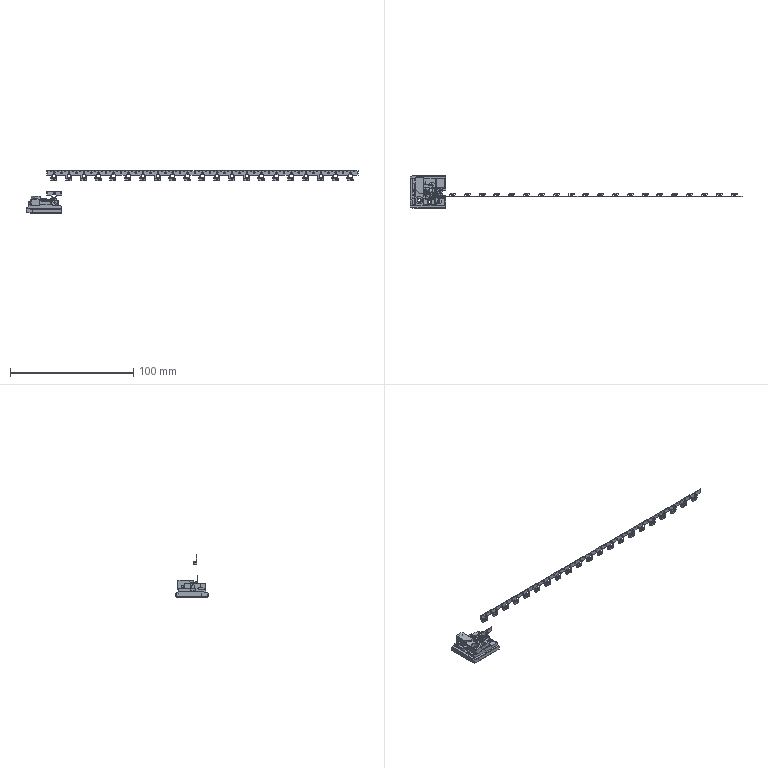Part | NX | 10 solids | 4586 faces | volume 5246 mm3 | plane 2703 | cylinder 1443 | torus 302 | spline 62 | sphere 48 | cone 28 | commonest cylinder face diameters 0.3 x352 0.2 x230 0.7 x118 1.3 x112 0.5 x111 0.4 x101